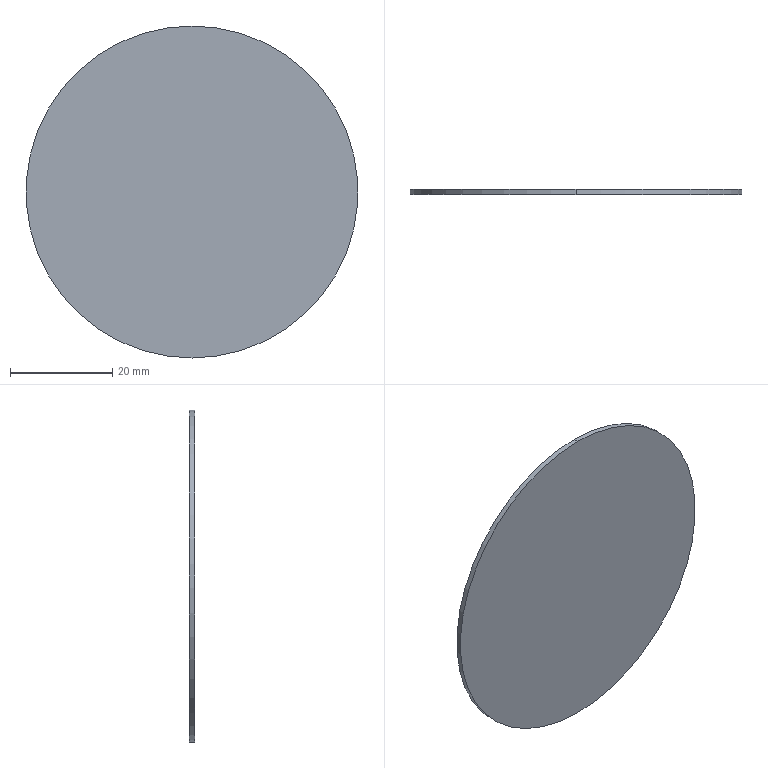Part | SolidWorks | features Extrusion 1 | 1 solid | 4 faces | box 65 x 1 x 65 mm | volume 3318 mm3 | cylinder 2 | plane 2 | commonest cylinder face diameters 65 x2
STEP:
#1=CARTESIAN_POINT('',(0.,1.,32.5));
#2=VERTEX_POINT('',#1);
#3=CARTESIAN_POINT('',(0.,1.,-32.5));
#4=VERTEX_POINT('',#3);
#5=CARTESIAN_POINT('',(0.,1.,0.));
#6=DIRECTION('',(0.,1.,0.));
#7=DIRECTION('',(0.,0.,1.));
#8=AXIS2_PLACEMENT_3D('',#5,#6,#7);
#9=CIRCLE('',#8,32.5);
#10=EDGE_CURVE('',#2,#4,#9,.T.);
#11=ORIENTED_EDGE('',*,*,#10,.F.);
#12=CARTESIAN_POINT('',(0.,0.,32.5));
#13=VERTEX_POINT('',#12);
#14=CARTESIAN_POINT('',(0.,1.,32.5));
#15=DIRECTION('',(0.,-1.,0.));
#16=VECTOR('',#15,1000.);
#17=LINE('',#14,#16);
#18=EDGE_CURVE('',#2,#13,#17,.T.);
#19=ORIENTED_EDGE('',*,*,#18,.T.);
#20=CARTESIAN_POINT('',(0.,0.,-32.5));
#21=VERTEX_POINT('',#20);
#22=CARTESIAN_POINT('',(0.,0.,0.));
#23=DIRECTION('',(0.,1.,0.));
#24=DIRECTION('',(0.,0.,1.));
#25=AXIS2_PLACEMENT_3D('',#22,#23,#24);
#26=CIRCLE('',#25,32.5);
#27=EDGE_CURVE('',#13,#21,#26,.T.);
#28=ORIENTED_EDGE('',*,*,#27,.T.);
#29=CARTESIAN_POINT('',(0.,1.,-32.5));
#30=DIRECTION('',(0.,-1.,0.));
#31=VECTOR('',#30,1000.);
#32=LINE('',#29,#31);
#33=EDGE_CURVE('',#4,#21,#32,.T.);
#34=ORIENTED_EDGE('',*,*,#33,.F.);
#35=EDGE_LOOP('',(#11,#19,#28,#34));
#36=FACE_OUTER_BOUND('',#35,.T.);
#37=CARTESIAN_POINT('',(0.,1.,0.));
#38=DIRECTION('',(0.,-1.,0.));
#39=DIRECTION('',(0.,0.,-1.));
#40=AXIS2_PLACEMENT_3D('',#37,#38,#39);
#41=CYLINDRICAL_SURFACE('',#40,32.5);
#42=ADVANCED_FACE('',(#36),#41,.T.);
#43=ORIENTED_EDGE('',*,*,#18,.F.);
#44=CARTESIAN_POINT('',(0.,1.,0.));
#45=DIRECTION('',(0.,1.,0.));
#46=DIRECTION('',(0.,0.,1.));
#47=AXIS2_PLACEMENT_3D('',#44,#45,#46);
#48=CIRCLE('',#47,32.5);
#49=EDGE_CURVE('',#4,#2,#48,.T.);
#50=ORIENTED_EDGE('',*,*,#49,.F.);
#51=ORIENTED_EDGE('',*,*,#33,.T.);
#52=CARTESIAN_POINT('',(0.,0.,0.));
#53=DIRECTION('',(0.,1.,0.));
#54=DIRECTION('',(0.,0.,1.));
#55=AXIS2_PLACEMENT_3D('',#52,#53,#54);
#56=CIRCLE('',#55,32.5);
#57=EDGE_CURVE('',#21,#13,#56,.T.);
#58=ORIENTED_EDGE('',*,*,#57,.T.);
#59=EDGE_LOOP('',(#43,#50,#51,#58));
#60=FACE_OUTER_BOUND('',#59,.T.);
#61=CARTESIAN_POINT('',(0.,1.,0.));
#62=DIRECTION('',(0.,-1.,0.));
#63=DIRECTION('',(0.,0.,-1.));
#64=AXIS2_PLACEMENT_3D('',#61,#62,#63);
#65=CYLINDRICAL_SURFACE('',#64,32.5);
#66=ADVANCED_FACE('',(#60),#65,.T.);
#67=ORIENTED_EDGE('',*,*,#49,.T.);
#68=ORIENTED_EDGE('',*,*,#10,.T.);
#69=EDGE_LOOP('',(#67,#68));
#70=FACE_OUTER_BOUND('',#69,.T.);
#71=CARTESIAN_POINT('',(0.,1.,0.));
#72=DIRECTION('',(0.,1.,0.));
#73=DIRECTION('',(0.,0.,1.));
#74=AXIS2_PLACEMENT_3D('',#71,#72,#73);
#75=PLANE('',#74);
#76=ADVANCED_FACE('',(#70),#75,.T.);
#77=ORIENTED_EDGE('',*,*,#57,.F.);
#78=ORIENTED_EDGE('',*,*,#27,.F.);
#79=EDGE_LOOP('',(#77,#78));
#80=FACE_OUTER_BOUND('',#79,.T.);
#81=CARTESIAN_POINT('',(0.,0.,0.));
#82=DIRECTION('',(0.,1.,0.));
#83=DIRECTION('',(0.,0.,1.));
#84=AXIS2_PLACEMENT_3D('',#81,#82,#83);
#85=PLANE('',#84);
#86=ADVANCED_FACE('',(#80),#85,.F.);
#87=CLOSED_SHELL('',(#42,#66,#76,#86));
#88=MANIFOLD_SOLID_BREP('',#87);
#89=CARTESIAN_POINT('',(0.,0.,0.));
#90=DIRECTION('',(0.,0.,1.));
#91=DIRECTION('',(1.,0.,0.));
#92=AXIS2_PLACEMENT_3D('',#89,#90,#91);
#93=(LENGTH_UNIT()NAMED_UNIT(*)SI_UNIT(.MILLI.,.METRE.));
#94=UNCERTAINTY_MEASURE_WITH_UNIT(LENGTH_MEASURE(0.00001),#93,'','');
#95=(NAMED_UNIT(*)PLANE_ANGLE_UNIT()SI_UNIT($,.RADIAN.));
#96=(NAMED_UNIT(*)SI_UNIT($,.STERADIAN.)SOLID_ANGLE_UNIT());
#97=(GEOMETRIC_REPRESENTATION_CONTEXT(3)GLOBAL_UNCERTAINTY_ASSIGNED_CONTEXT((#94))GLOBAL_UNIT_ASSIGNED_CONTEXT((#93,#95,#96))REPRESENTATION_CONTEXT('',''));
#98=ADVANCED_BREP_SHAPE_REPRESENTATION('',(#88,#92),#97);